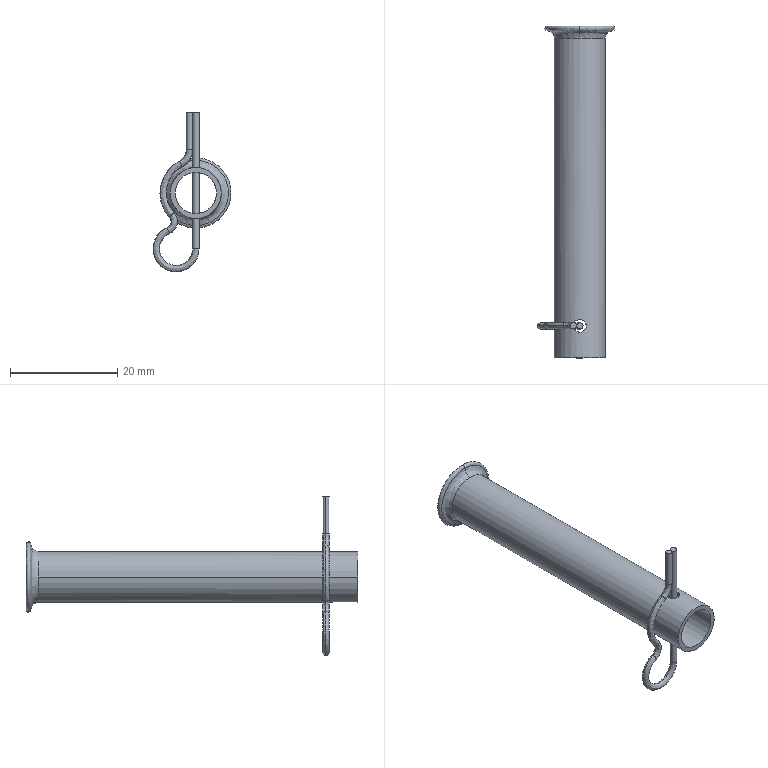Part | SolidWorks | features BaseBody 2 | 2 solids | 29 faces | box 14.556 x 62 x 29.835 mm | volume 1599 mm3 | spline 14 | cylinder 12 | plane 3 | commonest cylinder face diameters 1.2 x4 2.385 x4 7.747 x2 9.525 x2